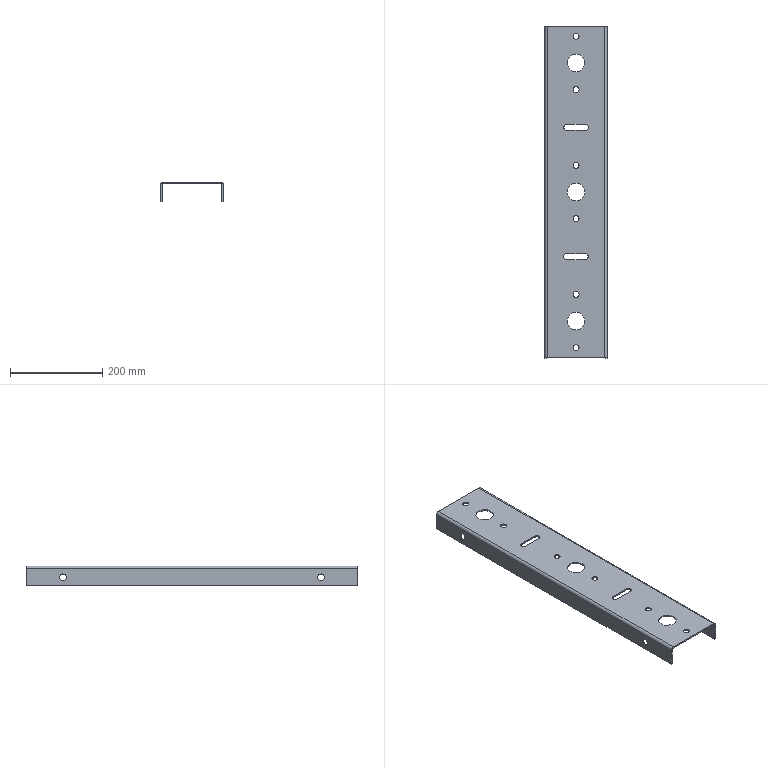Part | SolidWorks | features BaseBody 1 | 1 solid | 50 faces | box 136 x 720 x 43 mm | volume 439583 mm3 | cylinder 36 | plane 14 | commonest cylinder face diameters 13 x18 15 x8 38 x6 6 x2 12 x2